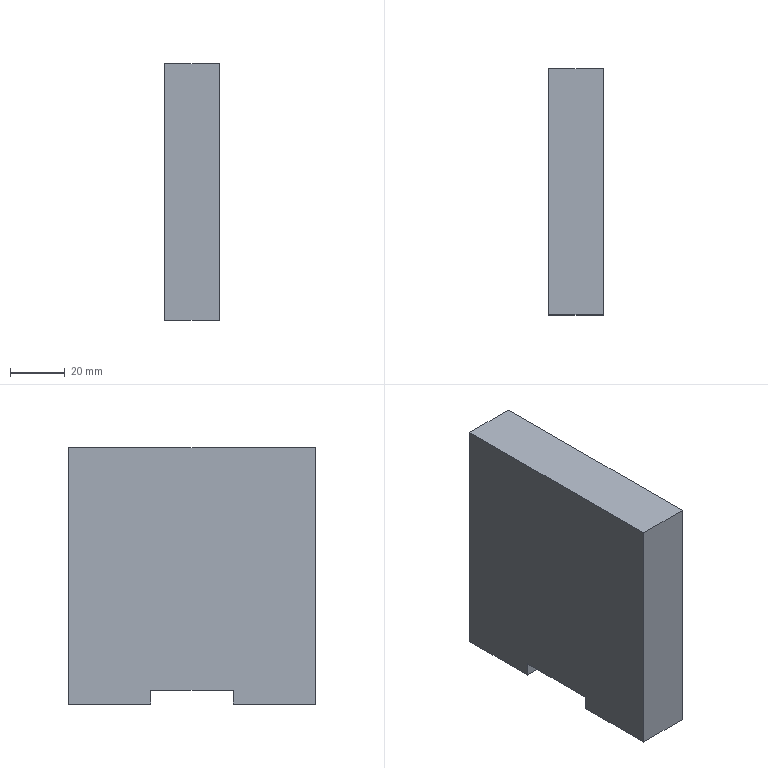Part | STEP file | PLC expansion module | 1 solid | 10 faces | box 20.1 x 90 x 93.7 mm | volume 166488 mm3 | plane 10
STEP:
#1=CARTESIAN_POINT('',(0.,0.,0.));
#2=DIRECTION('',(0.,0.,1.));
#3=DIRECTION('',(1.,0.,0.));
#4=AXIS2_PLACEMENT_3D('',#1,#2,#3);
#5=CARTESIAN_POINT('',(-10.05,-15.,0.));
#6=VERTEX_POINT('',#5);
#7=CARTESIAN_POINT('',(10.05,-15.,0.));
#8=VERTEX_POINT('',#7);
#9=CARTESIAN_POINT('',(-10.05,-15.,0.));
#10=DIRECTION('',(1.,0.,0.));
#11=VECTOR('',#10,1.);
#12=LINE('',#9,#11);
#13=CARTESIAN_POINT('',(0.,0.,0.));
#14=DIRECTION('',(0.,0.,-1.));
#15=DIRECTION('',(-1.,0.,0.));
#16=AXIS2_PLACEMENT_3D('',#13,#14,#15);
#17=PLANE('',#16);
#18=CARTESIAN_POINT('',(10.05,-15.));
#19=DIRECTION('',(-1.,0.));
#20=VECTOR('',#19,1.);
#21=LINE('',#18,#20);
#22=(GEOMETRIC_REPRESENTATION_CONTEXT(2)PARAMETRIC_REPRESENTATION_CONTEXT()REPRESENTATION_CONTEXT('',''));
#23=DEFINITIONAL_REPRESENTATION('',(#21),#22);
#24=PCURVE('',#17,#23);
#25=CARTESIAN_POINT('',(-10.05,-15.,0.));
#26=DIRECTION('',(0.,-1.,0.));
#27=DIRECTION('',(1.,0.,0.));
#28=AXIS2_PLACEMENT_3D('',#25,#26,#27);
#29=PLANE('',#28);
#30=CARTESIAN_POINT('',(0.,0.));
#31=DIRECTION('',(1.,0.));
#32=VECTOR('',#31,1.);
#33=LINE('',#30,#32);
#34=(GEOMETRIC_REPRESENTATION_CONTEXT(2)PARAMETRIC_REPRESENTATION_CONTEXT()REPRESENTATION_CONTEXT('',''));
#35=DEFINITIONAL_REPRESENTATION('',(#33),#34);
#36=PCURVE('',#29,#35);
#37=SURFACE_CURVE('',#12,(#24,#36),.PCURVE_S1.);
#38=EDGE_CURVE('',#6,#8,#37,.T.);
#39=ORIENTED_EDGE('',*,*,#38,.T.);
#40=CARTESIAN_POINT('',(10.05,-45.,0.));
#41=VERTEX_POINT('',#40);
#42=CARTESIAN_POINT('',(10.05,45.,0.));
#43=DIRECTION('',(0.,1.,0.));
#44=VECTOR('',#43,1.);
#45=LINE('',#42,#44);
#46=CARTESIAN_POINT('',(-10.05,45.));
#47=DIRECTION('',(0.,1.));
#48=VECTOR('',#47,1.);
#49=LINE('',#46,#48);
#50=(GEOMETRIC_REPRESENTATION_CONTEXT(2)PARAMETRIC_REPRESENTATION_CONTEXT()REPRESENTATION_CONTEXT('',''));
#51=DEFINITIONAL_REPRESENTATION('',(#49),#50);
#52=PCURVE('',#17,#51);
#53=CARTESIAN_POINT('',(10.05,45.,93.7));
#54=DIRECTION('',(-1.,0.,0.));
#55=DIRECTION('',(0.,-1.,0.));
#56=AXIS2_PLACEMENT_3D('',#53,#54,#55);
#57=PLANE('',#56);
#58=CARTESIAN_POINT('',(0.,-93.7));
#59=DIRECTION('',(-1.,0.));
#60=VECTOR('',#59,1.);
#61=LINE('',#58,#60);
#62=(GEOMETRIC_REPRESENTATION_CONTEXT(2)PARAMETRIC_REPRESENTATION_CONTEXT()REPRESENTATION_CONTEXT('',''));
#63=DEFINITIONAL_REPRESENTATION('',(#61),#62);
#64=PCURVE('',#57,#63);
#65=SURFACE_CURVE('',#45,(#52,#64),.PCURVE_S1.);
#66=EDGE_CURVE('',#41,#8,#65,.T.);
#67=ORIENTED_EDGE('',*,*,#66,.F.);
#68=CARTESIAN_POINT('',(-10.05,-45.,0.));
#69=VERTEX_POINT('',#68);
#70=CARTESIAN_POINT('',(10.05,-45.,0.));
#71=DIRECTION('',(1.,0.,0.));
#72=VECTOR('',#71,1.);
#73=LINE('',#70,#72);
#74=CARTESIAN_POINT('',(-10.05,-45.));
#75=DIRECTION('',(-1.,0.));
#76=VECTOR('',#75,1.);
#77=LINE('',#74,#76);
#78=(GEOMETRIC_REPRESENTATION_CONTEXT(2)PARAMETRIC_REPRESENTATION_CONTEXT()REPRESENTATION_CONTEXT('',''));
#79=DEFINITIONAL_REPRESENTATION('',(#77),#78);
#80=PCURVE('',#17,#79);
#81=CARTESIAN_POINT('',(10.05,-45.,93.7));
#82=DIRECTION('',(0.,1.,0.));
#83=DIRECTION('',(-1.,0.,0.));
#84=AXIS2_PLACEMENT_3D('',#81,#82,#83);
#85=PLANE('',#84);
#86=CARTESIAN_POINT('',(0.,-93.7));
#87=DIRECTION('',(-1.,0.));
#88=VECTOR('',#87,1.);
#89=LINE('',#86,#88);
#90=(GEOMETRIC_REPRESENTATION_CONTEXT(2)PARAMETRIC_REPRESENTATION_CONTEXT()REPRESENTATION_CONTEXT('',''));
#91=DEFINITIONAL_REPRESENTATION('',(#89),#90);
#92=PCURVE('',#85,#91);
#93=SURFACE_CURVE('',#73,(#80,#92),.PCURVE_S1.);
#94=EDGE_CURVE('',#69,#41,#93,.T.);
#95=ORIENTED_EDGE('',*,*,#94,.F.);
#96=CARTESIAN_POINT('',(-10.05,45.,0.));
#97=DIRECTION('',(0.,-1.,0.));
#98=VECTOR('',#97,1.);
#99=LINE('',#96,#98);
#100=CARTESIAN_POINT('',(10.05,45.));
#101=DIRECTION('',(0.,-1.));
#102=VECTOR('',#101,1.);
#103=LINE('',#100,#102);
#104=(GEOMETRIC_REPRESENTATION_CONTEXT(2)PARAMETRIC_REPRESENTATION_CONTEXT()REPRESENTATION_CONTEXT('',''));
#105=DEFINITIONAL_REPRESENTATION('',(#103),#104);
#106=PCURVE('',#17,#105);
#107=CARTESIAN_POINT('',(-10.05,45.,93.7));
#108=DIRECTION('',(1.,0.,0.));
#109=DIRECTION('',(0.,1.,0.));
#110=AXIS2_PLACEMENT_3D('',#107,#108,#109);
#111=PLANE('',#110);
#112=CARTESIAN_POINT('',(0.,-93.7));
#113=DIRECTION('',(-1.,0.));
#114=VECTOR('',#113,1.);
#115=LINE('',#112,#114);
#116=(GEOMETRIC_REPRESENTATION_CONTEXT(2)PARAMETRIC_REPRESENTATION_CONTEXT()REPRESENTATION_CONTEXT('',''));
#117=DEFINITIONAL_REPRESENTATION('',(#115),#116);
#118=PCURVE('',#111,#117);
#119=SURFACE_CURVE('',#99,(#106,#118),.PCURVE_S1.);
#120=EDGE_CURVE('',#6,#69,#119,.T.);
#121=ORIENTED_EDGE('',*,*,#120,.F.);
#122=EDGE_LOOP('',(#39,#67,#95,#121));
#123=FACE_BOUND('',#122,.T.);
#124=ADVANCED_FACE('',(#123),#17,.T.);
#125=CARTESIAN_POINT('',(-10.05,15.,5.));
#126=VERTEX_POINT('',#125);
#127=CARTESIAN_POINT('',(-10.05,-15.,5.));
#128=VERTEX_POINT('',#127);
#129=CARTESIAN_POINT('',(-10.05,15.,5.));
#130=DIRECTION('',(0.,-1.,0.));
#131=VECTOR('',#130,1.);
#132=LINE('',#129,#131);
#133=CARTESIAN_POINT('',(-30.,-88.7));
#134=DIRECTION('',(-1.,0.));
#135=VECTOR('',#134,1.);
#136=LINE('',#133,#135);
#137=(GEOMETRIC_REPRESENTATION_CONTEXT(2)PARAMETRIC_REPRESENTATION_CONTEXT()REPRESENTATION_CONTEXT('',''));
#138=DEFINITIONAL_REPRESENTATION('',(#136),#137);
#139=PCURVE('',#111,#138);
#140=CARTESIAN_POINT('',(-10.05,15.,5.));
#141=DIRECTION('',(0.,0.,1.));
#142=DIRECTION('',(0.,-1.,0.));
#143=AXIS2_PLACEMENT_3D('',#140,#141,#142);
#144=PLANE('',#143);
#145=CARTESIAN_POINT('',(0.,0.));
#146=DIRECTION('',(1.,0.));
#147=VECTOR('',#146,1.);
#148=LINE('',#145,#147);
#149=(GEOMETRIC_REPRESENTATION_CONTEXT(2)PARAMETRIC_REPRESENTATION_CONTEXT()REPRESENTATION_CONTEXT('',''));
#150=DEFINITIONAL_REPRESENTATION('',(#148),#149);
#151=PCURVE('',#144,#150);
#152=SURFACE_CURVE('',#132,(#139,#151),.PCURVE_S1.);
#153=EDGE_CURVE('',#126,#128,#152,.T.);
#154=ORIENTED_EDGE('',*,*,#153,.T.);
#155=CARTESIAN_POINT('',(-10.05,-15.,0.));
#156=DIRECTION('',(0.,0.,-1.));
#157=VECTOR('',#156,1.);
#158=LINE('',#155,#157);
#159=CARTESIAN_POINT('',(-60.,-93.7));
#160=DIRECTION('',(0.,-1.));
#161=VECTOR('',#160,1.);
#162=LINE('',#159,#161);
#163=(GEOMETRIC_REPRESENTATION_CONTEXT(2)PARAMETRIC_REPRESENTATION_CONTEXT()REPRESENTATION_CONTEXT('',''));
#164=DEFINITIONAL_REPRESENTATION('',(#162),#163);
#165=PCURVE('',#111,#164);
#166=CARTESIAN_POINT('',(0.,0.));
#167=DIRECTION('',(0.,-1.));
#168=VECTOR('',#167,1.);
#169=LINE('',#166,#168);
#170=(GEOMETRIC_REPRESENTATION_CONTEXT(2)PARAMETRIC_REPRESENTATION_CONTEXT()REPRESENTATION_CONTEXT('',''));
#171=DEFINITIONAL_REPRESENTATION('',(#169),#170);
#172=PCURVE('',#29,#171);
#173=SURFACE_CURVE('',#158,(#165,#172),.PCURVE_S1.);
#174=EDGE_CURVE('',#128,#6,#173,.T.);
#175=ORIENTED_EDGE('',*,*,#174,.T.);
#176=ORIENTED_EDGE('',*,*,#120,.T.);
#177=CARTESIAN_POINT('',(-10.05,-45.,93.7));
#178=VERTEX_POINT('',#177);
#179=CARTESIAN_POINT('',(-10.05,-45.,93.7));
#180=DIRECTION('',(0.,0.,-1.));
#181=VECTOR('',#180,1.);
#182=LINE('',#179,#181);
#183=CARTESIAN_POINT('',(-90.,0.));
#184=DIRECTION('',(0.,-1.));
#185=VECTOR('',#184,1.);
#186=LINE('',#183,#185);
#187=(GEOMETRIC_REPRESENTATION_CONTEXT(2)PARAMETRIC_REPRESENTATION_CONTEXT()REPRESENTATION_CONTEXT('',''));
#188=DEFINITIONAL_REPRESENTATION('',(#186),#187);
#189=PCURVE('',#111,#188);
#190=CARTESIAN_POINT('',(20.1,0.));
#191=DIRECTION('',(0.,-1.));
#192=VECTOR('',#191,1.);
#193=LINE('',#190,#192);
#194=(GEOMETRIC_REPRESENTATION_CONTEXT(2)PARAMETRIC_REPRESENTATION_CONTEXT()REPRESENTATION_CONTEXT('',''));
#195=DEFINITIONAL_REPRESENTATION('',(#193),#194);
#196=PCURVE('',#85,#195);
#197=SURFACE_CURVE('',#182,(#189,#196),.PCURVE_S1.);
#198=EDGE_CURVE('',#178,#69,#197,.T.);
#199=ORIENTED_EDGE('',*,*,#198,.F.);
#200=CARTESIAN_POINT('',(-10.05,45.,93.7));
#201=VERTEX_POINT('',#200);
#202=CARTESIAN_POINT('',(-10.05,45.,93.7));
#203=DIRECTION('',(0.,-1.,0.));
#204=VECTOR('',#203,1.);
#205=LINE('',#202,#204);
#206=CARTESIAN_POINT('',(0.,0.));
#207=DIRECTION('',(-1.,0.));
#208=VECTOR('',#207,1.);
#209=LINE('',#206,#208);
#210=(GEOMETRIC_REPRESENTATION_CONTEXT(2)PARAMETRIC_REPRESENTATION_CONTEXT()REPRESENTATION_CONTEXT('',''));
#211=DEFINITIONAL_REPRESENTATION('',(#209),#210);
#212=PCURVE('',#111,#211);
#213=CARTESIAN_POINT('',(0.,0.,93.7));
#214=DIRECTION('',(0.,0.,-1.));
#215=DIRECTION('',(-1.,0.,0.));
#216=AXIS2_PLACEMENT_3D('',#213,#214,#215);
#217=PLANE('',#216);
#218=CARTESIAN_POINT('',(10.05,45.));
#219=DIRECTION('',(0.,-1.));
#220=VECTOR('',#219,1.);
#221=LINE('',#218,#220);
#222=(GEOMETRIC_REPRESENTATION_CONTEXT(2)PARAMETRIC_REPRESENTATION_CONTEXT()REPRESENTATION_CONTEXT('',''));
#223=DEFINITIONAL_REPRESENTATION('',(#221),#222);
#224=PCURVE('',#217,#223);
#225=SURFACE_CURVE('',#205,(#212,#224),.PCURVE_S1.);
#226=EDGE_CURVE('',#201,#178,#225,.T.);
#227=ORIENTED_EDGE('',*,*,#226,.F.);
#228=CARTESIAN_POINT('',(-10.05,45.,0.));
#229=VERTEX_POINT('',#228);
#230=CARTESIAN_POINT('',(-10.05,45.,93.7));
#231=DIRECTION('',(0.,0.,-1.));
#232=VECTOR('',#231,1.);
#233=LINE('',#230,#232);
#234=CARTESIAN_POINT('',(0.,0.));
#235=DIRECTION('',(0.,-1.));
#236=VECTOR('',#235,1.);
#237=LINE('',#234,#236);
#238=(GEOMETRIC_REPRESENTATION_CONTEXT(2)PARAMETRIC_REPRESENTATION_CONTEXT()REPRESENTATION_CONTEXT('',''));
#239=DEFINITIONAL_REPRESENTATION('',(#237),#238);
#240=PCURVE('',#111,#239);
#241=CARTESIAN_POINT('',(10.05,45.,93.7));
#242=DIRECTION('',(0.,-1.,0.));
#243=DIRECTION('',(1.,0.,0.));
#244=AXIS2_PLACEMENT_3D('',#241,#242,#243);
#245=PLANE('',#244);
#246=CARTESIAN_POINT('',(-20.1,0.));
#247=DIRECTION('',(0.,-1.));
#248=VECTOR('',#247,1.);
#249=LINE('',#246,#248);
#250=(GEOMETRIC_REPRESENTATION_CONTEXT(2)PARAMETRIC_REPRESENTATION_CONTEXT()REPRESENTATION_CONTEXT('',''));
#251=DEFINITIONAL_REPRESENTATION('',(#249),#250);
#252=PCURVE('',#245,#251);
#253=SURFACE_CURVE('',#233,(#240,#252),.PCURVE_S1.);
#254=EDGE_CURVE('',#201,#229,#253,.T.);
#255=ORIENTED_EDGE('',*,*,#254,.T.);
#256=CARTESIAN_POINT('',(-10.05,15.,0.));
#257=VERTEX_POINT('',#256);
#258=CARTESIAN_POINT('',(-10.05,45.,0.));
#259=DIRECTION('',(0.,-1.,0.));
#260=VECTOR('',#259,1.);
#261=LINE('',#258,#260);
#262=CARTESIAN_POINT('',(0.,-93.7));
#263=DIRECTION('',(-1.,0.));
#264=VECTOR('',#263,1.);
#265=LINE('',#262,#264);
#266=(GEOMETRIC_REPRESENTATION_CONTEXT(2)PARAMETRIC_REPRESENTATION_CONTEXT()REPRESENTATION_CONTEXT('',''));
#267=DEFINITIONAL_REPRESENTATION('',(#265),#266);
#268=PCURVE('',#111,#267);
#269=CARTESIAN_POINT('',(0.,0.,0.));
#270=DIRECTION('',(0.,0.,-1.));
#271=DIRECTION('',(-1.,0.,0.));
#272=AXIS2_PLACEMENT_3D('',#269,#270,#271);
#273=PLANE('',#272);
#274=CARTESIAN_POINT('',(10.05,45.));
#275=DIRECTION('',(0.,-1.));
#276=VECTOR('',#275,1.);
#277=LINE('',#274,#276);
#278=(GEOMETRIC_REPRESENTATION_CONTEXT(2)PARAMETRIC_REPRESENTATION_CONTEXT()REPRESENTATION_CONTEXT('',''));
#279=DEFINITIONAL_REPRESENTATION('',(#277),#278);
#280=PCURVE('',#273,#279);
#281=SURFACE_CURVE('',#261,(#268,#280),.PCURVE_S1.);
#282=EDGE_CURVE('',#229,#257,#281,.T.);
#283=ORIENTED_EDGE('',*,*,#282,.T.);
#284=CARTESIAN_POINT('',(-10.05,15.,0.));
#285=DIRECTION('',(0.,0.,1.));
#286=VECTOR('',#285,1.);
#287=LINE('',#284,#286);
#288=CARTESIAN_POINT('',(-30.,-93.7));
#289=DIRECTION('',(0.,1.));
#290=VECTOR('',#289,1.);
#291=LINE('',#288,#290);
#292=(GEOMETRIC_REPRESENTATION_CONTEXT(2)PARAMETRIC_REPRESENTATION_CONTEXT()REPRESENTATION_CONTEXT('',''));
#293=DEFINITIONAL_REPRESENTATION('',(#291),#292);
#294=PCURVE('',#111,#293);
#295=CARTESIAN_POINT('',(-10.05,15.,0.));
#296=DIRECTION('',(0.,1.,0.));
#297=DIRECTION('',(-1.,0.,0.));
#298=AXIS2_PLACEMENT_3D('',#295,#296,#297);
#299=PLANE('',#298);
#300=CARTESIAN_POINT('',(0.,0.));
#301=DIRECTION('',(0.,1.));
#302=VECTOR('',#301,1.);
#303=LINE('',#300,#302);
#304=(GEOMETRIC_REPRESENTATION_CONTEXT(2)PARAMETRIC_REPRESENTATION_CONTEXT()REPRESENTATION_CONTEXT('',''));
#305=DEFINITIONAL_REPRESENTATION('',(#303),#304);
#306=PCURVE('',#299,#305);
#307=SURFACE_CURVE('',#287,(#294,#306),.PCURVE_S1.);
#308=EDGE_CURVE('',#257,#126,#307,.T.);
#309=ORIENTED_EDGE('',*,*,#308,.T.);
#310=EDGE_LOOP('',(#154,#175,#176,#199,#227,#255,#283,#309));
#311=FACE_BOUND('',#310,.T.);
#312=ADVANCED_FACE('',(#311),#111,.F.);
#313=ORIENTED_EDGE('',*,*,#94,.T.);
#314=CARTESIAN_POINT('',(10.05,-45.,93.7));
#315=VERTEX_POINT('',#314);
#316=CARTESIAN_POINT('',(10.05,-45.,93.7));
#317=DIRECTION('',(0.,0.,-1.));
#318=VECTOR('',#317,1.);
#319=LINE('',#316,#318);
#320=CARTESIAN_POINT('',(0.,0.));
#321=DIRECTION('',(0.,-1.));
#322=VECTOR('',#321,1.);
#323=LINE('',#320,#322);
#324=(GEOMETRIC_REPRESENTATION_CONTEXT(2)PARAMETRIC_REPRESENTATION_CONTEXT()REPRESENTATION_CONTEXT('',''));
#325=DEFINITIONAL_REPRESENTATION('',(#323),#324);
#326=PCURVE('',#85,#325);
#327=CARTESIAN_POINT('',(90.,0.));
#328=DIRECTION('',(0.,-1.));
#329=VECTOR('',#328,1.);
#330=LINE('',#327,#329);
#331=(GEOMETRIC_REPRESENTATION_CONTEXT(2)PARAMETRIC_REPRESENTATION_CONTEXT()REPRESENTATION_CONTEXT('',''));
#332=DEFINITIONAL_REPRESENTATION('',(#330),#331);
#333=PCURVE('',#57,#332);
#334=SURFACE_CURVE('',#319,(#326,#333),.PCURVE_S1.);
#335=EDGE_CURVE('',#315,#41,#334,.T.);
#336=ORIENTED_EDGE('',*,*,#335,.F.);
#337=CARTESIAN_POINT('',(10.05,-45.,93.7));
#338=DIRECTION('',(1.,0.,0.));
#339=VECTOR('',#338,1.);
#340=LINE('',#337,#339);
#341=CARTESIAN_POINT('',(0.,0.));
#342=DIRECTION('',(-1.,0.));
#343=VECTOR('',#342,1.);
#344=LINE('',#341,#343);
#345=(GEOMETRIC_REPRESENTATION_CONTEXT(2)PARAMETRIC_REPRESENTATION_CONTEXT()REPRESENTATION_CONTEXT('',''));
#346=DEFINITIONAL_REPRESENTATION('',(#344),#345);
#347=PCURVE('',#85,#346);
#348=CARTESIAN_POINT('',(-10.05,-45.));
#349=DIRECTION('',(-1.,0.));
#350=VECTOR('',#349,1.);
#351=LINE('',#348,#350);
#352=(GEOMETRIC_REPRESENTATION_CONTEXT(2)PARAMETRIC_REPRESENTATION_CONTEXT()REPRESENTATION_CONTEXT('',''));
#353=DEFINITIONAL_REPRESENTATION('',(#351),#352);
#354=PCURVE('',#217,#353);
#355=SURFACE_CURVE('',#340,(#347,#354),.PCURVE_S1.);
#356=EDGE_CURVE('',#178,#315,#355,.T.);
#357=ORIENTED_EDGE('',*,*,#356,.F.);
#358=ORIENTED_EDGE('',*,*,#198,.T.);
#359=EDGE_LOOP('',(#313,#336,#357,#358));
#360=FACE_BOUND('',#359,.T.);
#361=ADVANCED_FACE('',(#360),#85,.F.);
#362=ORIENTED_EDGE('',*,*,#66,.T.);
#363=CARTESIAN_POINT('',(10.05,-15.,5.));
#364=VERTEX_POINT('',#363);
#365=CARTESIAN_POINT('',(10.05,-15.,0.));
#366=DIRECTION('',(0.,0.,-1.));
#367=VECTOR('',#366,1.);
#368=LINE('',#365,#367);
#369=CARTESIAN_POINT('',(60.,-93.7));
#370=DIRECTION('',(0.,-1.));
#371=VECTOR('',#370,1.);
#372=LINE('',#369,#371);
#373=(GEOMETRIC_REPRESENTATION_CONTEXT(2)PARAMETRIC_REPRESENTATION_CONTEXT()REPRESENTATION_CONTEXT('',''));
#374=DEFINITIONAL_REPRESENTATION('',(#372),#373);
#375=PCURVE('',#57,#374);
#376=CARTESIAN_POINT('',(20.1,0.));
#377=DIRECTION('',(0.,-1.));
#378=VECTOR('',#377,1.);
#379=LINE('',#376,#378);
#380=(GEOMETRIC_REPRESENTATION_CONTEXT(2)PARAMETRIC_REPRESENTATION_CONTEXT()REPRESENTATION_CONTEXT('',''));
#381=DEFINITIONAL_REPRESENTATION('',(#379),#380);
#382=PCURVE('',#29,#381);
#383=SURFACE_CURVE('',#368,(#375,#382),.PCURVE_S1.);
#384=EDGE_CURVE('',#364,#8,#383,.T.);
#385=ORIENTED_EDGE('',*,*,#384,.F.);
#386=CARTESIAN_POINT('',(10.05,15.,5.));
#387=VERTEX_POINT('',#386);
#388=CARTESIAN_POINT('',(10.05,15.,5.));
#389=DIRECTION('',(0.,-1.,0.));
#390=VECTOR('',#389,1.);
#391=LINE('',#388,#390);
#392=CARTESIAN_POINT('',(30.,-88.7));
#393=DIRECTION('',(1.,0.));
#394=VECTOR('',#393,1.);
#395=LINE('',#392,#394);
#396=(GEOMETRIC_REPRESENTATION_CONTEXT(2)PARAMETRIC_REPRESENTATION_CONTEXT()REPRESENTATION_CONTEXT('',''));
#397=DEFINITIONAL_REPRESENTATION('',(#395),#396);
#398=PCURVE('',#57,#397);
#399=CARTESIAN_POINT('',(0.,20.1));
#400=DIRECTION('',(1.,0.));
#401=VECTOR('',#400,1.);
#402=LINE('',#399,#401);
#403=(GEOMETRIC_REPRESENTATION_CONTEXT(2)PARAMETRIC_REPRESENTATION_CONTEXT()REPRESENTATION_CONTEXT('',''));
#404=DEFINITIONAL_REPRESENTATION('',(#402),#403);
#405=PCURVE('',#144,#404);
#406=SURFACE_CURVE('',#391,(#398,#405),.PCURVE_S1.);
#407=EDGE_CURVE('',#387,#364,#406,.T.);
#408=ORIENTED_EDGE('',*,*,#407,.F.);
#409=CARTESIAN_POINT('',(10.05,15.,0.));
#410=VERTEX_POINT('',#409);
#411=CARTESIAN_POINT('',(10.05,15.,0.));
#412=DIRECTION('',(0.,0.,1.));
#413=VECTOR('',#412,1.);
#414=LINE('',#411,#413);
#415=CARTESIAN_POINT('',(30.,-93.7));
#416=DIRECTION('',(0.,1.));
#417=VECTOR('',#416,1.);
#418=LINE('',#415,#417);
#419=(GEOMETRIC_REPRESENTATION_CONTEXT(2)PARAMETRIC_REPRESENTATION_CONTEXT()REPRESENTATION_CONTEXT('',''));
#420=DEFINITIONAL_REPRESENTATION('',(#418),#419);
#421=PCURVE('',#57,#420);
#422=CARTESIAN_POINT('',(-20.1,0.));
#423=DIRECTION('',(0.,1.));
#424=VECTOR('',#423,1.);
#425=LINE('',#422,#424);
#426=(GEOMETRIC_REPRESENTATION_CONTEXT(2)PARAMETRIC_REPRESENTATION_CONTEXT()REPRESENTATION_CONTEXT('',''));
#427=DEFINITIONAL_REPRESENTATION('',(#425),#426);
#428=PCURVE('',#299,#427);
#429=SURFACE_CURVE('',#414,(#421,#428),.PCURVE_S1.);
#430=EDGE_CURVE('',#410,#387,#429,.T.);
#431=ORIENTED_EDGE('',*,*,#430,.F.);
#432=CARTESIAN_POINT('',(10.05,45.,0.));
#433=VERTEX_POINT('',#432);
#434=CARTESIAN_POINT('',(10.05,45.,0.));
#435=DIRECTION('',(0.,1.,0.));
#436=VECTOR('',#435,1.);
#437=LINE('',#434,#436);
#438=CARTESIAN_POINT('',(0.,-93.7));
#439=DIRECTION('',(-1.,0.));
#440=VECTOR('',#439,1.);
#441=LINE('',#438,#440);
#442=(GEOMETRIC_REPRESENTATION_CONTEXT(2)PARAMETRIC_REPRESENTATION_CONTEXT()REPRESENTATION_CONTEXT('',''));
#443=DEFINITIONAL_REPRESENTATION('',(#441),#442);
#444=PCURVE('',#57,#443);
#445=CARTESIAN_POINT('',(-10.05,45.));
#446=DIRECTION('',(0.,1.));
#447=VECTOR('',#446,1.);
#448=LINE('',#445,#447);
#449=(GEOMETRIC_REPRESENTATION_CONTEXT(2)PARAMETRIC_REPRESENTATION_CONTEXT()REPRESENTATION_CONTEXT('',''));
#450=DEFINITIONAL_REPRESENTATION('',(#448),#449);
#451=PCURVE('',#273,#450);
#452=SURFACE_CURVE('',#437,(#444,#451),.PCURVE_S1.);
#453=EDGE_CURVE('',#410,#433,#452,.T.);
#454=ORIENTED_EDGE('',*,*,#453,.T.);
#455=CARTESIAN_POINT('',(10.05,45.,93.7));
#456=VERTEX_POINT('',#455);
#457=CARTESIAN_POINT('',(10.05,45.,93.7));
#458=DIRECTION('',(0.,0.,-1.));
#459=VECTOR('',#458,1.);
#460=LINE('',#457,#459);
#461=CARTESIAN_POINT('',(0.,0.));
#462=DIRECTION('',(0.,-1.));
#463=VECTOR('',#462,1.);
#464=LINE('',#461,#463);
#465=(GEOMETRIC_REPRESENTATION_CONTEXT(2)PARAMETRIC_REPRESENTATION_CONTEXT()REPRESENTATION_CONTEXT('',''));
#466=DEFINITIONAL_REPRESENTATION('',(#464),#465);
#467=PCURVE('',#57,#466);
#468=CARTESIAN_POINT('',(0.,0.));
#469=DIRECTION('',(0.,-1.));
#470=VECTOR('',#469,1.);
#471=LINE('',#468,#470);
#472=(GEOMETRIC_REPRESENTATION_CONTEXT(2)PARAMETRIC_REPRESENTATION_CONTEXT()REPRESENTATION_CONTEXT('',''));
#473=DEFINITIONAL_REPRESENTATION('',(#471),#472);
#474=PCURVE('',#245,#473);
#475=SURFACE_CURVE('',#460,(#467,#474),.PCURVE_S1.);
#476=EDGE_CURVE('',#456,#433,#475,.T.);
#477=ORIENTED_EDGE('',*,*,#476,.F.);
#478=CARTESIAN_POINT('',(10.05,45.,93.7));
#479=DIRECTION('',(0.,1.,0.));
#480=VECTOR('',#479,1.);
#481=LINE('',#478,#480);
#482=CARTESIAN_POINT('',(0.,0.));
#483=DIRECTION('',(-1.,0.));
#484=VECTOR('',#483,1.);
#485=LINE('',#482,#484);
#486=(GEOMETRIC_REPRESENTATION_CONTEXT(2)PARAMETRIC_REPRESENTATION_CONTEXT()REPRESENTATION_CONTEXT('',''));
#487=DEFINITIONAL_REPRESENTATION('',(#485),#486);
#488=PCURVE('',#57,#487);
#489=CARTESIAN_POINT('',(-10.05,45.));
#490=DIRECTION('',(0.,1.));
#491=VECTOR('',#490,1.);
#492=LINE('',#489,#491);
#493=(GEOMETRIC_REPRESENTATION_CONTEXT(2)PARAMETRIC_REPRESENTATION_CONTEXT()REPRESENTATION_CONTEXT('',''));
#494=DEFINITIONAL_REPRESENTATION('',(#492),#493);
#495=PCURVE('',#217,#494);
#496=SURFACE_CURVE('',#481,(#488,#495),.PCURVE_S1.);
#497=EDGE_CURVE('',#315,#456,#496,.T.);
#498=ORIENTED_EDGE('',*,*,#497,.F.);
#499=ORIENTED_EDGE('',*,*,#335,.T.);
#500=EDGE_LOOP('',(#362,#385,#408,#431,#454,#477,#498,#499));
#501=FACE_BOUND('',#500,.T.);
#502=ADVANCED_FACE('',(#501),#57,.F.);
#503=CARTESIAN_POINT('',(10.05,45.,0.));
#504=DIRECTION('',(-1.,0.,0.));
#505=VECTOR('',#504,1.);
#506=LINE('',#503,#505);
#507=CARTESIAN_POINT('',(0.,-93.7));
#508=DIRECTION('',(-1.,0.));
#509=VECTOR('',#508,1.);
#510=LINE('',#507,#509);
#511=(GEOMETRIC_REPRESENTATION_CONTEXT(2)PARAMETRIC_REPRESENTATION_CONTEXT()REPRESENTATION_CONTEXT('',''));
#512=DEFINITIONAL_REPRESENTATION('',(#510),#511);
#513=PCURVE('',#245,#512);
#514=CARTESIAN_POINT('',(-10.05,45.));
#515=DIRECTION('',(1.,0.));
#516=VECTOR('',#515,1.);
#517=LINE('',#514,#516);
#518=(GEOMETRIC_REPRESENTATION_CONTEXT(2)PARAMETRIC_REPRESENTATION_CONTEXT()REPRESENTATION_CONTEXT('',''));
#519=DEFINITIONAL_REPRESENTATION('',(#517),#518);
#520=PCURVE('',#273,#519);
#521=SURFACE_CURVE('',#506,(#513,#520),.PCURVE_S1.);
#522=EDGE_CURVE('',#433,#229,#521,.T.);
#523=ORIENTED_EDGE('',*,*,#522,.T.);
#524=ORIENTED_EDGE('',*,*,#254,.F.);
#525=CARTESIAN_POINT('',(10.05,45.,93.7));
#526=DIRECTION('',(-1.,0.,0.));
#527=VECTOR('',#526,1.);
#528=LINE('',#525,#527);
#529=CARTESIAN_POINT('',(0.,0.));
#530=DIRECTION('',(-1.,0.));
#531=VECTOR('',#530,1.);
#532=LINE('',#529,#531);
#533=(GEOMETRIC_REPRESENTATION_CONTEXT(2)PARAMETRIC_REPRESENTATION_CONTEXT()REPRESENTATION_CONTEXT('',''));
#534=DEFINITIONAL_REPRESENTATION('',(#532),#533);
#535=PCURVE('',#245,#534);
#536=CARTESIAN_POINT('',(-10.05,45.));
#537=DIRECTION('',(1.,0.));
#538=VECTOR('',#537,1.);
#539=LINE('',#536,#538);
#540=(GEOMETRIC_REPRESENTATION_CONTEXT(2)PARAMETRIC_REPRESENTATION_CONTEXT()REPRESENTATION_CONTEXT('',''));
#541=DEFINITIONAL_REPRESENTATION('',(#539),#540);
#542=PCURVE('',#217,#541);
#543=SURFACE_CURVE('',#528,(#535,#542),.PCURVE_S1.);
#544=EDGE_CURVE('',#456,#201,#543,.T.);
#545=ORIENTED_EDGE('',*,*,#544,.F.);
#546=ORIENTED_EDGE('',*,*,#476,.T.);
#547=EDGE_LOOP('',(#523,#524,#545,#546));
#548=FACE_BOUND('',#547,.T.);
#549=ADVANCED_FACE('',(#548),#245,.F.);
#550=ORIENTED_EDGE('',*,*,#226,.T.);
#551=ORIENTED_EDGE('',*,*,#356,.T.);
#552=ORIENTED_EDGE('',*,*,#497,.T.);
#553=ORIENTED_EDGE('',*,*,#544,.T.);
#554=EDGE_LOOP('',(#550,#551,#552,#553));
#555=FACE_BOUND('',#554,.T.);
#556=ADVANCED_FACE('',(#555),#217,.F.);
#557=CARTESIAN_POINT('',(-10.05,15.,0.));
#558=DIRECTION('',(1.,0.,0.));
#559=VECTOR('',#558,1.);
#560=LINE('',#557,#559);
#561=CARTESIAN_POINT('',(10.05,15.));
#562=DIRECTION('',(-1.,0.));
#563=VECTOR('',#562,1.);
#564=LINE('',#561,#563);
#565=(GEOMETRIC_REPRESENTATION_CONTEXT(2)PARAMETRIC_REPRESENTATION_CONTEXT()REPRESENTATION_CONTEXT('',''));
#566=DEFINITIONAL_REPRESENTATION('',(#564),#565);
#567=PCURVE('',#273,#566);
#568=CARTESIAN_POINT('',(0.,0.));
#569=DIRECTION('',(-1.,0.));
#570=VECTOR('',#569,1.);
#571=LINE('',#568,#570);
#572=(GEOMETRIC_REPRESENTATION_CONTEXT(2)PARAMETRIC_REPRESENTATION_CONTEXT()REPRESENTATION_CONTEXT('',''));
#573=DEFINITIONAL_REPRESENTATION('',(#571),#572);
#574=PCURVE('',#299,#573);
#575=SURFACE_CURVE('',#560,(#567,#574),.PCURVE_S1.);
#576=EDGE_CURVE('',#257,#410,#575,.T.);
#577=ORIENTED_EDGE('',*,*,#576,.F.);
#578=ORIENTED_EDGE('',*,*,#282,.F.);
#579=ORIENTED_EDGE('',*,*,#522,.F.);
#580=ORIENTED_EDGE('',*,*,#453,.F.);
#581=EDGE_LOOP('',(#577,#578,#579,#580));
#582=FACE_BOUND('',#581,.T.);
#583=ADVANCED_FACE('',(#582),#273,.T.);
#584=ORIENTED_EDGE('',*,*,#384,.T.);
#585=ORIENTED_EDGE('',*,*,#38,.F.);
#586=ORIENTED_EDGE('',*,*,#174,.F.);
#587=CARTESIAN_POINT('',(-10.05,-15.,5.));
#588=DIRECTION('',(1.,0.,0.));
#589=VECTOR('',#588,1.);
#590=LINE('',#587,#589);
#591=CARTESIAN_POINT('',(0.,5.));
#592=DIRECTION('',(1.,0.));
#593=VECTOR('',#592,1.);
#594=LINE('',#591,#593);
#595=(GEOMETRIC_REPRESENTATION_CONTEXT(2)PARAMETRIC_REPRESENTATION_CONTEXT()REPRESENTATION_CONTEXT('',''));
#596=DEFINITIONAL_REPRESENTATION('',(#594),#595);
#597=PCURVE('',#29,#596);
#598=CARTESIAN_POINT('',(30.,0.));
#599=DIRECTION('',(0.,1.));
#600=VECTOR('',#599,1.);
#601=LINE('',#598,#600);
#602=(GEOMETRIC_REPRESENTATION_CONTEXT(2)PARAMETRIC_REPRESENTATION_CONTEXT()REPRESENTATION_CONTEXT('',''));
#603=DEFINITIONAL_REPRESENTATION('',(#601),#602);
#604=PCURVE('',#144,#603);
#605=SURFACE_CURVE('',#590,(#597,#604),.PCURVE_S1.);
#606=EDGE_CURVE('',#128,#364,#605,.T.);
#607=ORIENTED_EDGE('',*,*,#606,.T.);
#608=EDGE_LOOP('',(#584,#585,#586,#607));
#609=FACE_BOUND('',#608,.T.);
#610=ADVANCED_FACE('',(#609),#29,.F.);
#611=ORIENTED_EDGE('',*,*,#407,.T.);
#612=ORIENTED_EDGE('',*,*,#606,.F.);
#613=ORIENTED_EDGE('',*,*,#153,.F.);
#614=CARTESIAN_POINT('',(-10.05,15.,5.));
#615=DIRECTION('',(1.,0.,0.));
#616=VECTOR('',#615,1.);
#617=LINE('',#614,#616);
#618=CARTESIAN_POINT('',(0.,0.));
#619=DIRECTION('',(0.,1.));
#620=VECTOR('',#619,1.);
#621=LINE('',#618,#620);
#622=(GEOMETRIC_REPRESENTATION_CONTEXT(2)PARAMETRIC_REPRESENTATION_CONTEXT()REPRESENTATION_CONTEXT('',''));
#623=DEFINITIONAL_REPRESENTATION('',(#621),#622);
#624=PCURVE('',#144,#623);
#625=CARTESIAN_POINT('',(0.,5.));
#626=DIRECTION('',(-1.,0.));
#627=VECTOR('',#626,1.);
#628=LINE('',#625,#627);
#629=(GEOMETRIC_REPRESENTATION_CONTEXT(2)PARAMETRIC_REPRESENTATION_CONTEXT()REPRESENTATION_CONTEXT('',''));
#630=DEFINITIONAL_REPRESENTATION('',(#628),#629);
#631=PCURVE('',#299,#630);
#632=SURFACE_CURVE('',#617,(#624,#631),.PCURVE_S1.);
#633=EDGE_CURVE('',#126,#387,#632,.T.);
#634=ORIENTED_EDGE('',*,*,#633,.T.);
#635=EDGE_LOOP('',(#611,#612,#613,#634));
#636=FACE_BOUND('',#635,.T.);
#637=ADVANCED_FACE('',(#636),#144,.F.);
#638=ORIENTED_EDGE('',*,*,#430,.T.);
#639=ORIENTED_EDGE('',*,*,#633,.F.);
#640=ORIENTED_EDGE('',*,*,#308,.F.);
#641=ORIENTED_EDGE('',*,*,#576,.T.);
#642=EDGE_LOOP('',(#638,#639,#640,#641));
#643=FACE_BOUND('',#642,.T.);
#644=ADVANCED_FACE('',(#643),#299,.F.);
#645=CLOSED_SHELL('',(#124,#312,#361,#502,#549,#556,#583,#610,#637,#644));
#646=MANIFOLD_SOLID_BREP('',#645);
#647=(LENGTH_UNIT()NAMED_UNIT(*)SI_UNIT(.MILLI.,.METRE.));
#648=UNCERTAINTY_MEASURE_WITH_UNIT(LENGTH_MEASURE(0.0000001),#647,'','');
#649=(NAMED_UNIT(*)PLANE_ANGLE_UNIT()SI_UNIT($,.RADIAN.));
#650=(NAMED_UNIT(*)SI_UNIT($,.STERADIAN.)SOLID_ANGLE_UNIT());
#651=(GEOMETRIC_REPRESENTATION_CONTEXT(3)GLOBAL_UNCERTAINTY_ASSIGNED_CONTEXT((#648))GLOBAL_UNIT_ASSIGNED_CONTEXT((#647,#649,#650))REPRESENTATION_CONTEXT('',''));
#652=ADVANCED_BREP_SHAPE_REPRESENTATION('',(#4,#646),#651);